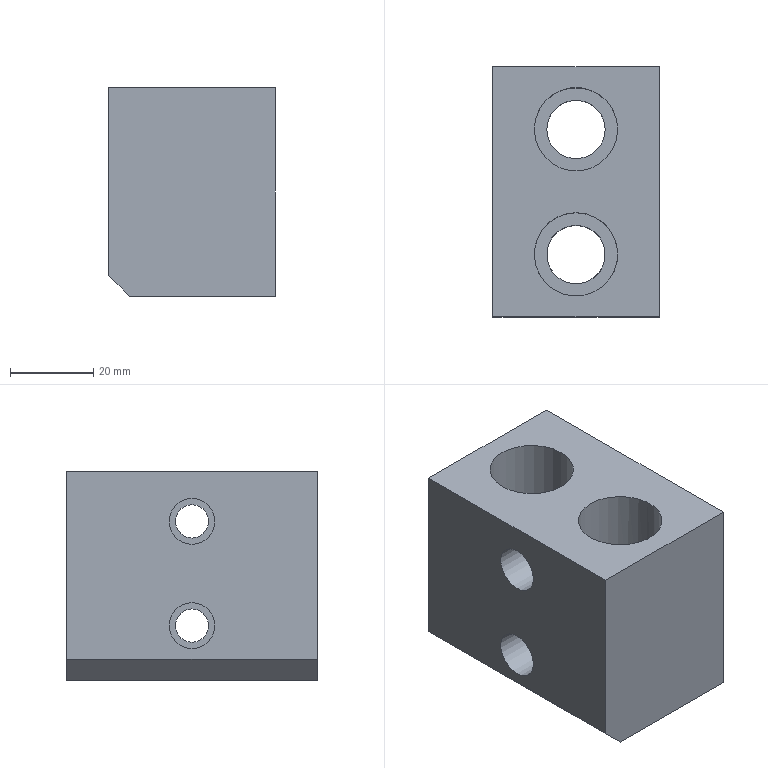Part | NX | features solid 2 | 1 solid | 19 faces | box 40 x 60 x 50 mm | volume 90929 mm3 | plane 11 | cylinder 8 | commonest cylinder face diameters 8 x2 11 x2 14 x2 20 x2
STEP:
#1=CARTESIAN_POINT('',(280.,365.,-457.9));
#2=VERTEX_POINT('',#1);
#3=CARTESIAN_POINT('',(280.,365.,-461.9));
#4=DIRECTION('',(-1.,0.,0.));
#5=DIRECTION('',(0.,0.,1.));
#6=AXIS2_PLACEMENT_3D('',#3,#4,#5);
#7=CIRCLE('',#6,4.);
#8=EDGE_CURVE('',#2,#2,#7,.F.);
#9=ORIENTED_EDGE('',*,*,#8,.F.);
#10=EDGE_LOOP('',(#9));
#11=FACE_BOUND('',#10,.T.);
#12=CARTESIAN_POINT('',(280.,365.,-432.9));
#13=VERTEX_POINT('',#12);
#14=CARTESIAN_POINT('',(280.,365.,-436.9));
#15=DIRECTION('',(-1.,0.,0.));
#16=DIRECTION('',(0.,0.,1.));
#17=AXIS2_PLACEMENT_3D('',#14,#15,#16);
#18=CIRCLE('',#17,4.);
#19=EDGE_CURVE('',#13,#13,#18,.F.);
#20=ORIENTED_EDGE('',*,*,#19,.F.);
#21=EDGE_LOOP('',(#20));
#22=FACE_BOUND('',#21,.T.);
#23=CARTESIAN_POINT('',(280.,335.,-475.));
#24=VERTEX_POINT('',#23);
#25=CARTESIAN_POINT('',(280.,395.,-475.));
#26=VERTEX_POINT('',#25);
#27=CARTESIAN_POINT('',(280.,335.,-475.));
#28=DIRECTION('',(0.,-1.,0.));
#29=VECTOR('',#28,1000.);
#30=LINE('',#27,#29);
#31=EDGE_CURVE('',#24,#26,#30,.F.);
#32=ORIENTED_EDGE('',*,*,#31,.T.);
#33=CARTESIAN_POINT('',(280.,395.,-425.));
#34=VERTEX_POINT('',#33);
#35=CARTESIAN_POINT('',(280.,395.,-425.));
#36=DIRECTION('',(0.,0.,-1.));
#37=VECTOR('',#36,1000.);
#38=LINE('',#35,#37);
#39=EDGE_CURVE('',#34,#26,#38,.T.);
#40=ORIENTED_EDGE('',*,*,#39,.F.);
#41=CARTESIAN_POINT('',(280.,335.,-425.));
#42=VERTEX_POINT('',#41);
#43=CARTESIAN_POINT('',(280.,335.,-425.));
#44=DIRECTION('',(0.,1.,0.));
#45=VECTOR('',#44,1000.);
#46=LINE('',#43,#45);
#47=EDGE_CURVE('',#42,#34,#46,.T.);
#48=ORIENTED_EDGE('',*,*,#47,.F.);
#49=CARTESIAN_POINT('',(280.,335.,-425.));
#50=DIRECTION('',(0.,0.,1.));
#51=VECTOR('',#50,1000.);
#52=LINE('',#49,#51);
#53=EDGE_CURVE('',#42,#24,#52,.F.);
#54=ORIENTED_EDGE('',*,*,#53,.T.);
#55=EDGE_LOOP('',(#32,#40,#48,#54));
#56=FACE_BOUND('',#55,.T.);
#57=CARTESIAN_POINT('',(280.,335.,-425.));
#58=DIRECTION('',(-1.,0.,0.));
#59=DIRECTION('',(0.,0.,-1.));
#60=AXIS2_PLACEMENT_3D('',#57,#58,#59);
#61=PLANE('',#60);
#62=ADVANCED_FACE('',(#11,#22,#56),#61,.F.);
#63=CARTESIAN_POINT('',(240.,365.,-456.4));
#64=VERTEX_POINT('',#63);
#65=CARTESIAN_POINT('',(240.,365.,-461.9));
#66=DIRECTION('',(-1.,0.,0.));
#67=DIRECTION('',(0.,0.,1.));
#68=AXIS2_PLACEMENT_3D('',#65,#66,#67);
#69=CIRCLE('',#68,5.5);
#70=EDGE_CURVE('',#64,#64,#69,.T.);
#71=ORIENTED_EDGE('',*,*,#70,.F.);
#72=EDGE_LOOP('',(#71));
#73=FACE_BOUND('',#72,.T.);
#74=CARTESIAN_POINT('',(240.,365.,-431.4));
#75=VERTEX_POINT('',#74);
#76=CARTESIAN_POINT('',(240.,365.,-436.9));
#77=DIRECTION('',(-1.,0.,0.));
#78=DIRECTION('',(0.,0.,1.));
#79=AXIS2_PLACEMENT_3D('',#76,#77,#78);
#80=CIRCLE('',#79,5.5);
#81=EDGE_CURVE('',#75,#75,#80,.T.);
#82=ORIENTED_EDGE('',*,*,#81,.F.);
#83=EDGE_LOOP('',(#82));
#84=FACE_BOUND('',#83,.T.);
#85=CARTESIAN_POINT('',(240.,335.,-425.));
#86=VERTEX_POINT('',#85);
#87=CARTESIAN_POINT('',(240.,335.,-470.));
#88=VERTEX_POINT('',#87);
#89=CARTESIAN_POINT('',(240.,335.,-425.));
#90=DIRECTION('',(0.,0.,-1.));
#91=VECTOR('',#90,1000.);
#92=LINE('',#89,#91);
#93=EDGE_CURVE('',#86,#88,#92,.T.);
#94=ORIENTED_EDGE('',*,*,#93,.F.);
#95=CARTESIAN_POINT('',(240.,395.,-425.));
#96=VERTEX_POINT('',#95);
#97=CARTESIAN_POINT('',(240.,335.,-425.));
#98=DIRECTION('',(0.,1.,0.));
#99=VECTOR('',#98,1000.);
#100=LINE('',#97,#99);
#101=EDGE_CURVE('',#86,#96,#100,.T.);
#102=ORIENTED_EDGE('',*,*,#101,.T.);
#103=CARTESIAN_POINT('',(240.,395.,-470.));
#104=VERTEX_POINT('',#103);
#105=CARTESIAN_POINT('',(240.,395.,-425.));
#106=DIRECTION('',(0.,0.,-1.));
#107=VECTOR('',#106,1000.);
#108=LINE('',#105,#107);
#109=EDGE_CURVE('',#96,#104,#108,.T.);
#110=ORIENTED_EDGE('',*,*,#109,.T.);
#111=CARTESIAN_POINT('',(240.,395.,-470.));
#112=DIRECTION('',(0.,1.,0.));
#113=VECTOR('',#112,1000.);
#114=LINE('',#111,#113);
#115=EDGE_CURVE('',#88,#104,#114,.T.);
#116=ORIENTED_EDGE('',*,*,#115,.F.);
#117=EDGE_LOOP('',(#94,#102,#110,#116));
#118=FACE_BOUND('',#117,.T.);
#119=CARTESIAN_POINT('',(240.,335.,-425.));
#120=DIRECTION('',(-1.,0.,0.));
#121=DIRECTION('',(0.,0.,-1.));
#122=AXIS2_PLACEMENT_3D('',#119,#120,#121);
#123=PLANE('',#122);
#124=ADVANCED_FACE('',(#73,#84,#118),#123,.T.);
#125=CARTESIAN_POINT('',(245.,335.,-475.));
#126=VERTEX_POINT('',#125);
#127=CARTESIAN_POINT('',(270.,335.,-475.));
#128=DIRECTION('',(1.,0.,0.));
#129=VECTOR('',#128,1000.);
#130=LINE('',#127,#129);
#131=EDGE_CURVE('',#126,#24,#130,.T.);
#132=ORIENTED_EDGE('',*,*,#131,.T.);
#133=ORIENTED_EDGE('',*,*,#53,.F.);
#134=CARTESIAN_POINT('',(270.,335.,-425.));
#135=DIRECTION('',(-1.,0.,0.));
#136=VECTOR('',#135,1000.);
#137=LINE('',#134,#136);
#138=EDGE_CURVE('',#86,#42,#137,.F.);
#139=ORIENTED_EDGE('',*,*,#138,.F.);
#140=ORIENTED_EDGE('',*,*,#93,.T.);
#141=CARTESIAN_POINT('',(240.,335.,-470.));
#142=DIRECTION('',(-0.7071,0.,0.7071));
#143=VECTOR('',#142,1000.);
#144=LINE('',#141,#143);
#145=EDGE_CURVE('',#126,#88,#144,.T.);
#146=ORIENTED_EDGE('',*,*,#145,.F.);
#147=EDGE_LOOP('',(#132,#133,#139,#140,#146));
#148=FACE_BOUND('',#147,.T.);
#149=CARTESIAN_POINT('',(270.,335.,-425.));
#150=DIRECTION('',(0.,-1.,0.));
#151=DIRECTION('',(0.,0.,-1.));
#152=AXIS2_PLACEMENT_3D('',#149,#150,#151);
#153=PLANE('',#152);
#154=ADVANCED_FACE('',(#148),#153,.T.);
#155=CARTESIAN_POINT('',(253.,380.,-475.));
#156=VERTEX_POINT('',#155);
#157=CARTESIAN_POINT('',(260.,380.,-475.));
#158=DIRECTION('',(0.,0.,-1.));
#159=DIRECTION('',(-1.,0.,0.));
#160=AXIS2_PLACEMENT_3D('',#157,#158,#159);
#161=CIRCLE('',#160,7.);
#162=EDGE_CURVE('',#156,#156,#161,.T.);
#163=ORIENTED_EDGE('',*,*,#162,.F.);
#164=EDGE_LOOP('',(#163));
#165=FACE_BOUND('',#164,.T.);
#166=CARTESIAN_POINT('',(245.,395.,-475.));
#167=VERTEX_POINT('',#166);
#168=CARTESIAN_POINT('',(270.,395.,-475.));
#169=DIRECTION('',(-1.,0.,0.));
#170=VECTOR('',#169,1000.);
#171=LINE('',#168,#170);
#172=EDGE_CURVE('',#167,#26,#171,.F.);
#173=ORIENTED_EDGE('',*,*,#172,.T.);
#174=ORIENTED_EDGE('',*,*,#31,.F.);
#175=ORIENTED_EDGE('',*,*,#131,.F.);
#176=CARTESIAN_POINT('',(245.,335.,-475.));
#177=DIRECTION('',(0.,1.,0.));
#178=VECTOR('',#177,1000.);
#179=LINE('',#176,#178);
#180=EDGE_CURVE('',#167,#126,#179,.F.);
#181=ORIENTED_EDGE('',*,*,#180,.F.);
#182=EDGE_LOOP('',(#173,#174,#175,#181));
#183=FACE_BOUND('',#182,.T.);
#184=CARTESIAN_POINT('',(253.,350.,-475.));
#185=VERTEX_POINT('',#184);
#186=CARTESIAN_POINT('',(260.,350.,-475.));
#187=DIRECTION('',(0.,0.,-1.));
#188=DIRECTION('',(-1.,0.,0.));
#189=AXIS2_PLACEMENT_3D('',#186,#187,#188);
#190=CIRCLE('',#189,7.);
#191=EDGE_CURVE('',#185,#185,#190,.T.);
#192=ORIENTED_EDGE('',*,*,#191,.F.);
#193=EDGE_LOOP('',(#192));
#194=FACE_BOUND('',#193,.T.);
#195=CARTESIAN_POINT('',(270.,335.,-475.));
#196=DIRECTION('',(0.,0.,-1.));
#197=DIRECTION('',(0.,1.,0.));
#198=AXIS2_PLACEMENT_3D('',#195,#196,#197);
#199=PLANE('',#198);
#200=ADVANCED_FACE('',(#165,#183,#194),#199,.T.);
#201=ORIENTED_EDGE('',*,*,#109,.F.);
#202=CARTESIAN_POINT('',(270.,395.,-425.));
#203=DIRECTION('',(1.,0.,0.));
#204=VECTOR('',#203,1000.);
#205=LINE('',#202,#204);
#206=EDGE_CURVE('',#96,#34,#205,.T.);
#207=ORIENTED_EDGE('',*,*,#206,.T.);
#208=ORIENTED_EDGE('',*,*,#39,.T.);
#209=ORIENTED_EDGE('',*,*,#172,.F.);
#210=CARTESIAN_POINT('',(240.,395.,-470.));
#211=DIRECTION('',(-0.7071,0.,0.7071));
#212=VECTOR('',#211,1000.);
#213=LINE('',#210,#212);
#214=EDGE_CURVE('',#104,#167,#213,.F.);
#215=ORIENTED_EDGE('',*,*,#214,.F.);
#216=EDGE_LOOP('',(#201,#207,#208,#209,#215));
#217=FACE_BOUND('',#216,.T.);
#218=CARTESIAN_POINT('',(270.,395.,-425.));
#219=DIRECTION('',(0.,-1.,0.));
#220=DIRECTION('',(0.,0.,-1.));
#221=AXIS2_PLACEMENT_3D('',#218,#219,#220);
#222=PLANE('',#221);
#223=ADVANCED_FACE('',(#217),#222,.F.);
#224=CARTESIAN_POINT('',(250.,380.,-425.));
#225=VERTEX_POINT('',#224);
#226=CARTESIAN_POINT('',(260.,380.,-425.));
#227=DIRECTION('',(0.,0.,-1.));
#228=DIRECTION('',(-1.,0.,0.));
#229=AXIS2_PLACEMENT_3D('',#226,#227,#228);
#230=CIRCLE('',#229,10.);
#231=EDGE_CURVE('',#225,#225,#230,.F.);
#232=ORIENTED_EDGE('',*,*,#231,.F.);
#233=EDGE_LOOP('',(#232));
#234=FACE_BOUND('',#233,.T.);
#235=CARTESIAN_POINT('',(250.,350.,-425.));
#236=VERTEX_POINT('',#235);
#237=CARTESIAN_POINT('',(260.,350.,-425.));
#238=DIRECTION('',(0.,0.,-1.));
#239=DIRECTION('',(-1.,0.,0.));
#240=AXIS2_PLACEMENT_3D('',#237,#238,#239);
#241=CIRCLE('',#240,10.);
#242=EDGE_CURVE('',#236,#236,#241,.F.);
#243=ORIENTED_EDGE('',*,*,#242,.F.);
#244=EDGE_LOOP('',(#243));
#245=FACE_BOUND('',#244,.T.);
#246=ORIENTED_EDGE('',*,*,#101,.F.);
#247=ORIENTED_EDGE('',*,*,#138,.T.);
#248=ORIENTED_EDGE('',*,*,#47,.T.);
#249=ORIENTED_EDGE('',*,*,#206,.F.);
#250=EDGE_LOOP('',(#246,#247,#248,#249));
#251=FACE_BOUND('',#250,.T.);
#252=CARTESIAN_POINT('',(270.,335.,-425.));
#253=DIRECTION('',(0.,0.,-1.));
#254=DIRECTION('',(0.,1.,0.));
#255=AXIS2_PLACEMENT_3D('',#252,#253,#254);
#256=PLANE('',#255);
#257=ADVANCED_FACE('',(#234,#245,#251),#256,.F.);
#258=CARTESIAN_POINT('',(260.,357.,-450.));
#259=VERTEX_POINT('',#258);
#260=CARTESIAN_POINT('',(260.,350.,-450.));
#261=DIRECTION('',(0.,0.,1.));
#262=DIRECTION('',(0.,1.,0.));
#263=AXIS2_PLACEMENT_3D('',#260,#261,#262);
#264=CIRCLE('',#263,7.);
#265=EDGE_CURVE('',#259,#259,#264,.T.);
#266=ORIENTED_EDGE('',*,*,#265,.T.);
#267=EDGE_LOOP('',(#266));
#268=FACE_BOUND('',#267,.T.);
#269=ORIENTED_EDGE('',*,*,#191,.T.);
#270=EDGE_LOOP('',(#269));
#271=FACE_BOUND('',#270,.T.);
#272=CARTESIAN_POINT('',(260.,350.,-505.));
#273=DIRECTION('',(0.,0.,-1.));
#274=DIRECTION('',(1.,0.,0.));
#275=AXIS2_PLACEMENT_3D('',#272,#273,#274);
#276=CYLINDRICAL_SURFACE('',#275,7.);
#277=ADVANCED_FACE('',(#268,#271),#276,.F.);
#278=ORIENTED_EDGE('',*,*,#265,.F.);
#279=EDGE_LOOP('',(#278));
#280=FACE_BOUND('',#279,.T.);
#281=CARTESIAN_POINT('',(260.,360.,-450.));
#282=VERTEX_POINT('',#281);
#283=CARTESIAN_POINT('',(260.,350.,-450.));
#284=DIRECTION('',(0.,0.,1.));
#285=DIRECTION('',(0.,1.,0.));
#286=AXIS2_PLACEMENT_3D('',#283,#284,#285);
#287=CIRCLE('',#286,10.);
#288=EDGE_CURVE('',#282,#282,#287,.T.);
#289=ORIENTED_EDGE('',*,*,#288,.T.);
#290=EDGE_LOOP('',(#289));
#291=FACE_BOUND('',#290,.T.);
#292=CARTESIAN_POINT('',(260.,380.,-450.));
#293=DIRECTION('',(0.,0.,-1.));
#294=DIRECTION('',(1.,0.,0.));
#295=AXIS2_PLACEMENT_3D('',#292,#293,#294);
#296=PLANE('',#295);
#297=ADVANCED_FACE('',(#280,#291),#296,.F.);
#298=ORIENTED_EDGE('',*,*,#288,.F.);
#299=EDGE_LOOP('',(#298));
#300=FACE_BOUND('',#299,.T.);
#301=ORIENTED_EDGE('',*,*,#242,.T.);
#302=EDGE_LOOP('',(#301));
#303=FACE_BOUND('',#302,.T.);
#304=CARTESIAN_POINT('',(260.,350.,-425.));
#305=DIRECTION('',(0.,0.,-1.));
#306=DIRECTION('',(1.,0.,0.));
#307=AXIS2_PLACEMENT_3D('',#304,#305,#306);
#308=CYLINDRICAL_SURFACE('',#307,10.);
#309=ADVANCED_FACE('',(#300,#303),#308,.F.);
#310=CARTESIAN_POINT('',(253.,380.,-450.));
#311=VERTEX_POINT('',#310);
#312=CARTESIAN_POINT('',(260.,380.,-450.));
#313=DIRECTION('',(0.,0.,-1.));
#314=DIRECTION('',(-1.,0.,0.));
#315=AXIS2_PLACEMENT_3D('',#312,#313,#314);
#316=CIRCLE('',#315,7.);
#317=EDGE_CURVE('',#311,#311,#316,.F.);
#318=ORIENTED_EDGE('',*,*,#317,.T.);
#319=EDGE_LOOP('',(#318));
#320=FACE_BOUND('',#319,.T.);
#321=ORIENTED_EDGE('',*,*,#162,.T.);
#322=EDGE_LOOP('',(#321));
#323=FACE_BOUND('',#322,.T.);
#324=CARTESIAN_POINT('',(260.,380.,-505.));
#325=DIRECTION('',(0.,0.,-1.));
#326=DIRECTION('',(1.,0.,0.));
#327=AXIS2_PLACEMENT_3D('',#324,#325,#326);
#328=CYLINDRICAL_SURFACE('',#327,7.);
#329=ADVANCED_FACE('',(#320,#323),#328,.F.);
#330=ORIENTED_EDGE('',*,*,#317,.F.);
#331=EDGE_LOOP('',(#330));
#332=FACE_BOUND('',#331,.T.);
#333=CARTESIAN_POINT('',(250.,380.,-450.));
#334=VERTEX_POINT('',#333);
#335=CARTESIAN_POINT('',(260.,380.,-450.));
#336=DIRECTION('',(0.,0.,-1.));
#337=DIRECTION('',(-1.,0.,0.));
#338=AXIS2_PLACEMENT_3D('',#335,#336,#337);
#339=CIRCLE('',#338,10.);
#340=EDGE_CURVE('',#334,#334,#339,.F.);
#341=ORIENTED_EDGE('',*,*,#340,.T.);
#342=EDGE_LOOP('',(#341));
#343=FACE_BOUND('',#342,.T.);
#344=CARTESIAN_POINT('',(260.,380.,-450.));
#345=DIRECTION('',(0.,0.,-1.));
#346=DIRECTION('',(1.,0.,0.));
#347=AXIS2_PLACEMENT_3D('',#344,#345,#346);
#348=PLANE('',#347);
#349=ADVANCED_FACE('',(#332,#343),#348,.F.);
#350=ORIENTED_EDGE('',*,*,#340,.F.);
#351=EDGE_LOOP('',(#350));
#352=FACE_BOUND('',#351,.T.);
#353=ORIENTED_EDGE('',*,*,#231,.T.);
#354=EDGE_LOOP('',(#353));
#355=FACE_BOUND('',#354,.T.);
#356=CARTESIAN_POINT('',(260.,380.,-425.));
#357=DIRECTION('',(0.,0.,-1.));
#358=DIRECTION('',(1.,0.,0.));
#359=AXIS2_PLACEMENT_3D('',#356,#357,#358);
#360=CYLINDRICAL_SURFACE('',#359,10.);
#361=ADVANCED_FACE('',(#352,#355),#360,.F.);
#362=CARTESIAN_POINT('',(250.,365.,-440.9));
#363=VERTEX_POINT('',#362);
#364=CARTESIAN_POINT('',(250.,365.,-436.9));
#365=DIRECTION('',(1.,0.,0.));
#366=DIRECTION('',(0.,0.,-1.));
#367=AXIS2_PLACEMENT_3D('',#364,#365,#366);
#368=CIRCLE('',#367,4.);
#369=EDGE_CURVE('',#363,#363,#368,.F.);
#370=ORIENTED_EDGE('',*,*,#369,.T.);
#371=EDGE_LOOP('',(#370));
#372=FACE_BOUND('',#371,.T.);
#373=ORIENTED_EDGE('',*,*,#19,.T.);
#374=EDGE_LOOP('',(#373));
#375=FACE_BOUND('',#374,.T.);
#376=CARTESIAN_POINT('',(290.,365.,-436.9));
#377=DIRECTION('',(1.,0.,0.));
#378=DIRECTION('',(0.,0.,1.));
#379=AXIS2_PLACEMENT_3D('',#376,#377,#378);
#380=CYLINDRICAL_SURFACE('',#379,4.);
#381=ADVANCED_FACE('',(#372,#375),#380,.F.);
#382=ORIENTED_EDGE('',*,*,#369,.F.);
#383=EDGE_LOOP('',(#382));
#384=FACE_BOUND('',#383,.T.);
#385=CARTESIAN_POINT('',(250.,365.,-442.4));
#386=VERTEX_POINT('',#385);
#387=CARTESIAN_POINT('',(250.,365.,-436.9));
#388=DIRECTION('',(1.,0.,0.));
#389=DIRECTION('',(0.,0.,-1.));
#390=AXIS2_PLACEMENT_3D('',#387,#388,#389);
#391=CIRCLE('',#390,5.5);
#392=EDGE_CURVE('',#386,#386,#391,.F.);
#393=ORIENTED_EDGE('',*,*,#392,.T.);
#394=EDGE_LOOP('',(#393));
#395=FACE_BOUND('',#394,.T.);
#396=CARTESIAN_POINT('',(250.,365.,-440.1));
#397=DIRECTION('',(1.,0.,0.));
#398=DIRECTION('',(0.,0.,1.));
#399=AXIS2_PLACEMENT_3D('',#396,#397,#398);
#400=PLANE('',#399);
#401=ADVANCED_FACE('',(#384,#395),#400,.F.);
#402=ORIENTED_EDGE('',*,*,#392,.F.);
#403=EDGE_LOOP('',(#402));
#404=FACE_BOUND('',#403,.T.);
#405=ORIENTED_EDGE('',*,*,#81,.T.);
#406=EDGE_LOOP('',(#405));
#407=FACE_BOUND('',#406,.T.);
#408=CARTESIAN_POINT('',(240.,365.,-436.9));
#409=DIRECTION('',(1.,0.,0.));
#410=DIRECTION('',(0.,0.,1.));
#411=AXIS2_PLACEMENT_3D('',#408,#409,#410);
#412=CYLINDRICAL_SURFACE('',#411,5.5);
#413=ADVANCED_FACE('',(#404,#407),#412,.F.);
#414=CARTESIAN_POINT('',(250.,365.,-465.9));
#415=VERTEX_POINT('',#414);
#416=CARTESIAN_POINT('',(250.,365.,-461.9));
#417=DIRECTION('',(1.,0.,0.));
#418=DIRECTION('',(0.,0.,-1.));
#419=AXIS2_PLACEMENT_3D('',#416,#417,#418);
#420=CIRCLE('',#419,4.);
#421=EDGE_CURVE('',#415,#415,#420,.F.);
#422=ORIENTED_EDGE('',*,*,#421,.T.);
#423=EDGE_LOOP('',(#422));
#424=FACE_BOUND('',#423,.T.);
#425=ORIENTED_EDGE('',*,*,#8,.T.);
#426=EDGE_LOOP('',(#425));
#427=FACE_BOUND('',#426,.T.);
#428=CARTESIAN_POINT('',(290.,365.,-461.9));
#429=DIRECTION('',(1.,0.,0.));
#430=DIRECTION('',(0.,0.,1.));
#431=AXIS2_PLACEMENT_3D('',#428,#429,#430);
#432=CYLINDRICAL_SURFACE('',#431,4.);
#433=ADVANCED_FACE('',(#424,#427),#432,.F.);
#434=ORIENTED_EDGE('',*,*,#421,.F.);
#435=EDGE_LOOP('',(#434));
#436=FACE_BOUND('',#435,.T.);
#437=CARTESIAN_POINT('',(250.,365.,-467.4));
#438=VERTEX_POINT('',#437);
#439=CARTESIAN_POINT('',(250.,365.,-461.9));
#440=DIRECTION('',(1.,0.,0.));
#441=DIRECTION('',(0.,0.,-1.));
#442=AXIS2_PLACEMENT_3D('',#439,#440,#441);
#443=CIRCLE('',#442,5.5);
#444=EDGE_CURVE('',#438,#438,#443,.F.);
#445=ORIENTED_EDGE('',*,*,#444,.T.);
#446=EDGE_LOOP('',(#445));
#447=FACE_BOUND('',#446,.T.);
#448=CARTESIAN_POINT('',(250.,365.,-465.1));
#449=DIRECTION('',(1.,0.,0.));
#450=DIRECTION('',(0.,0.,1.));
#451=AXIS2_PLACEMENT_3D('',#448,#449,#450);
#452=PLANE('',#451);
#453=ADVANCED_FACE('',(#436,#447),#452,.F.);
#454=ORIENTED_EDGE('',*,*,#444,.F.);
#455=EDGE_LOOP('',(#454));
#456=FACE_BOUND('',#455,.T.);
#457=ORIENTED_EDGE('',*,*,#70,.T.);
#458=EDGE_LOOP('',(#457));
#459=FACE_BOUND('',#458,.T.);
#460=CARTESIAN_POINT('',(240.,365.,-461.9));
#461=DIRECTION('',(1.,0.,0.));
#462=DIRECTION('',(0.,0.,1.));
#463=AXIS2_PLACEMENT_3D('',#460,#461,#462);
#464=CYLINDRICAL_SURFACE('',#463,5.5);
#465=ADVANCED_FACE('',(#456,#459),#464,.F.);
#466=ORIENTED_EDGE('',*,*,#145,.T.);
#467=ORIENTED_EDGE('',*,*,#115,.T.);
#468=ORIENTED_EDGE('',*,*,#214,.T.);
#469=ORIENTED_EDGE('',*,*,#180,.T.);
#470=EDGE_LOOP('',(#466,#467,#468,#469));
#471=FACE_BOUND('',#470,.T.);
#472=CARTESIAN_POINT('',(240.,335.,-470.));
#473=DIRECTION('',(0.7071,0.,0.7071));
#474=DIRECTION('',(-0.7071,0.,0.7071));
#475=AXIS2_PLACEMENT_3D('',#472,#473,#474);
#476=PLANE('',#475);
#477=ADVANCED_FACE('',(#471),#476,.F.);
#478=CLOSED_SHELL('',(#62,#124,#154,#200,#223,#257,#277,#297,#309,#329,#349,#361,#381,#401,#413,#433,#453,#465,#477));
#479=MANIFOLD_SOLID_BREP('',#478);
#480=(LENGTH_UNIT()NAMED_UNIT(*)SI_UNIT(.MILLI.,.METRE.));
#481=UNCERTAINTY_MEASURE_WITH_UNIT(LENGTH_MEASURE(0.00001),#480,'','');
#482=(NAMED_UNIT(*)PLANE_ANGLE_UNIT()SI_UNIT($,.RADIAN.));
#483=(NAMED_UNIT(*)SI_UNIT($,.STERADIAN.)SOLID_ANGLE_UNIT());
#484=(GEOMETRIC_REPRESENTATION_CONTEXT(3)GLOBAL_UNCERTAINTY_ASSIGNED_CONTEXT((#481))GLOBAL_UNIT_ASSIGNED_CONTEXT((#480,#482,#483))REPRESENTATION_CONTEXT('',''));
#485=ADVANCED_BREP_SHAPE_REPRESENTATION('',(#479),#484);